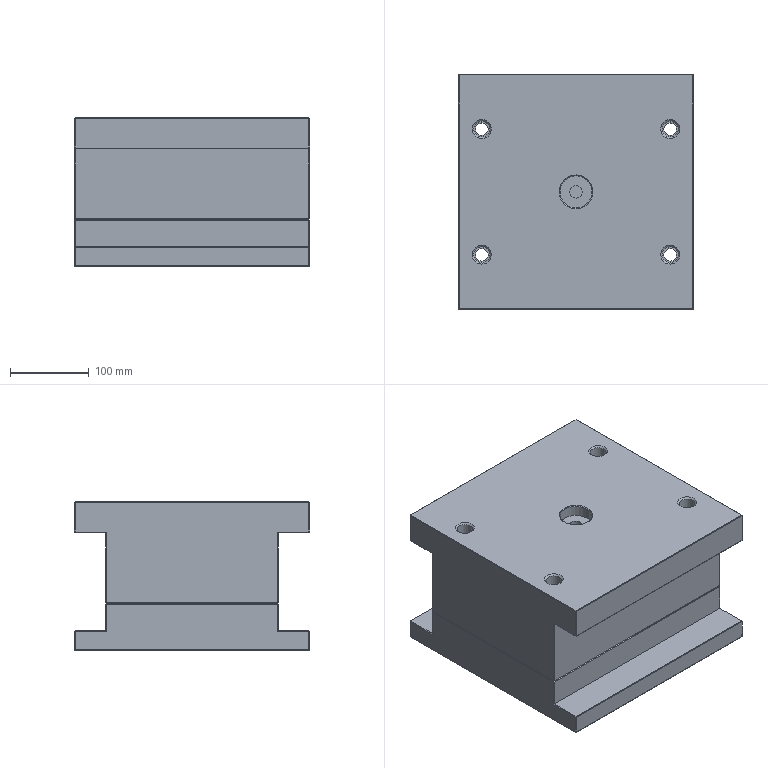NC program | NX | posted with a generic post | part box 300 x 300 x 190 mm
Lines 1 to 898 of 6235:
N10 G17 G21 G94 G90
(CAVITY_MILL , TOOL : D25R5)
N12 T02 M6
N14 G54
N16 G17 G0 G90 X-9.973 Y-6.502 S1000 M3
N18 G43 Z30. H2
N20 Z1.5
N22 G94 G1 X-9.815 Y-6.752 Z1.484 F1000.
N24 X-8.984 Y-7.824 Z1.413
N26 X-8.037 Y-8.794 Z1.342
N28 X-6.985 Y-9.651 Z1.271
N30 X-5.843 Y-10.382 Z1.2
N32 X-4.625 Y-10.979 Z1.129
N34 X-3.347 Y-11.434 Z1.058
N36 X-2.026 Y-11.74 Z0.987
N38 X-0.678 Y-11.894 Z0.916
N40 X0.678 Z0.845
N42 X2.026 Y-11.74 Z0.774
N44 X3.347 Y-11.434 Z0.703
N46 X4.625 Y-10.979 Z0.631
N48 X5.843 Y-10.382 Z0.56
N50 X6.985 Y-9.651 Z0.489
N52 X8.037 Y-8.794 Z0.418
N54 X8.984 Y-7.824 Z0.347
N56 X9.815 Y-6.752 Z0.276
N58 X10.335 Y-5.926 Z0.225
N60 X10.855 Y-4.909 Z0.165
N62 X11.276 Y-3.847 Z0.105
N64 X11.592 Y-2.749 Z0.045
N66 X11.802 Y-1.626 Z-0.015
N68 X11.904 Y-0.488 Z-0.074
N70 Y0. Z-0.1
N72 X2.154
N74 G3 X0. Y2.154 R2.154 F2000.
N76 X2.154 Y0. R-2.154
N78 G1 X11.904
N80 G3 X0. Y11.904 R11.904
N82 X11.904 Y0. R-11.904
N84 G1 X21.654
N86 G3 X0. Y21.654 R21.654
N88 X21.654 Y0. R-21.654
N90 G1 X31.404
N92 G3 X0. Y31.404 R31.404
N94 X31.404 Y0. R-31.404
N96 G1 X41.154
N98 G3 X0. Y41.154 R41.154
N100 X41.154 Y0. R-41.154
N102 X40.654 Y0.866 R1.
N104 G1 Z1.4
N106 G0 X-1.355 Y11.092
N108 G1 X-1.643 Y11.061 Z1.385 F1000.
N110 X-2.887 Y10.804 Z1.318
N112 X-4.095 Y10.406 Z1.252
N114 X-5.249 Y9.874 Z1.185
N116 X-6.336 Y9.215 Z1.118
N118 X-7.341 Y8.436 Z1.052
N120 X-8.251 Y7.549 Z0.985
N122 X-9.054 Y6.564 Z0.919
N124 X-9.74 Y5.494 Z0.852
N126 X-10.301 Y4.353 Z0.785
N128 X-10.728 Y3.156 Z0.719
N130 X-11.017 Y1.918 Z0.652
N132 X-11.164 Y0.655 Z0.585
N134 X-11.166 Y-0.616 Z0.519
N136 X-11.024 Y-1.879 Z0.452
N138 X-10.739 Y-3.118 Z0.386
N140 X-10.316 Y-4.317 Z0.319
N142 X-9.759 Y-5.46 Z0.252
N144 X-9.263 Y-6.265 Z0.203
N146 X-8.471 Y-7.301 Z0.134
N148 X-7.563 Y-8.238 Z0.066
N150 X-6.552 Y-9.062 Z-0.002
N152 X-5.452 Y-9.764 Z-0.071
N154 X-4.277 Y-10.332 Z-0.139
N156 X-3.045 Y-10.76 Z-0.207
N158 X-1.771 Y-11.042 Z-0.276
N160 X-0.473 Y-11.173 Z-0.344
N162 X0. Z-0.369
N164 Y-1.423
N166 G3 X1.423 Y0. R1.423 F2000.
N168 X0. Y-1.423 R-1.423
N170 G1 Y-11.173
N172 G3 X11.173 Y0. R11.173
N174 X0. Y-11.173 R-11.173
N176 G1 Y-20.923
N178 G3 X20.923 Y0. R20.923
N180 X0. Y-20.923 R-20.923
N182 G1 Y-30.673
N184 G3 X30.673 Y0. R30.673
N186 X0. Y-30.673 R-30.673
N188 G1 Y-40.423
N190 G3 X40.423 Y0. R40.423
N192 X0. Y-40.423 R-40.423
N194 X0.866 Y-39.923 R1.
N196 G1 Z1.131
N198 G0 X0.232 Y10.67
N200 G1 X0.115 Y10.676 Z1.125 F1000.
N202 X-0.674 Y10.655 Z1.083
N204 X-1.593 Y10.557 Z1.035
N206 X-2.857 Y10.287 Z0.967
N208 X-4.079 Y9.867 Z0.9
N210 X-5.241 Y9.302 Z0.832
N212 X-6.326 Y8.6 Z0.764
N214 X-7.319 Y7.773 Z0.696
N216 X-8.205 Y6.832 Z0.629
N218 X-8.97 Y5.79 Z0.561
N220 X-9.604 Y4.664 Z0.493
N222 X-10.097 Y3.469 Z0.425
N224 X-10.442 Y2.224 Z0.358
N226 X-10.635 Y0.946 Z0.29
N228 X-10.671 Y-0.346 Z0.222
N230 X-10.551 Y-1.633 Z0.155
N232 X-10.276 Y-2.895 Z0.087
N234 X-9.851 Y-4.116 Z0.019
N236 X-9.282 Y-5.276 Z-0.049
N238 X-8.791 Y-6.059 Z-0.097
N240 X-8.034 Y-7.032 Z-0.162
N242 X-7.17 Y-7.911 Z-0.226
N244 X-6.211 Y-8.684 Z-0.291
N246 X-5.168 Y-9.342 Z-0.355
N248 X-4.057 Y-9.876 Z-0.42
N250 X-2.892 Y-10.277 Z-0.485
N252 X-1.688 Y-10.542 Z-0.549
N254 X-0.462 Y-10.667 Z-0.614
N256 X0. Z-0.638
N258 Y-0.917
N260 G3 X0.917 Y0. R0.917 F2000.
N262 X0. Y-0.917 R-0.917
N264 G1 Y-10.667
N266 G3 X10.667 Y0. R10.667
N268 X0. Y-10.667 R-10.667
N270 G1 Y-20.417
N272 G3 X20.417 Y0. R20.417
N274 X0. Y-20.417 R-20.417
N276 G1 Y-30.167
N278 G3 X30.167 Y0. R30.167
N280 X0. Y-30.167 R-30.167
N282 G1 Y-39.917
N284 G3 X39.917 Y0. R39.917
N286 X0. Y-39.917 R-39.917
N288 X0.866 Y-39.417 R1.
N290 G1 Z0.862
N292 G0 X10.171 Y-1.473
N294 G1 X10.277 Y-0.246 Z0.797 F1000.
N296 X10.228 Y1.034 Z0.73
N298 X10.02 Y2.297 Z0.663
N300 X9.657 Y3.524 Z0.596
N302 X9.144 Y4.697 Z0.529
N304 X8.489 Y5.797 Z0.462
N306 X7.703 Y6.808 Z0.395
N308 X6.797 Y7.712 Z0.328
N310 X5.786 Y8.497 Z0.261
N312 X4.685 Y9.15 Z0.194
N314 X3.511 Y9.662 Z0.126
N316 X2.283 Y10.023 Z0.059
N318 X1.391 Y10.185 Z0.012
N320 X0.464 Y10.269 Z-0.037
N322 X-0.467 Z-0.086
N324 X-1.37 Y10.188 Z-0.133
N326 X-2.541 Y9.961 Z-0.196
N328 X-3.677 Y9.6 Z-0.258
N330 X-4.765 Y9.109 Z-0.321
N332 X-5.788 Y8.496 Z-0.383
N334 X-6.733 Y7.768 Z-0.446
N336 X-7.587 Y6.936 Z-0.508
N338 X-8.339 Y6.011 Z-0.571
N340 X-8.979 Y5.004 Z-0.633
N342 X-9.499 Y3.931 Z-0.696
N344 X-9.89 Y2.804 Z-0.758
N346 X-10.148 Y1.64 Z-0.821
N348 X-10.27 Y0.453 Z-0.883
N350 Y0. Z-0.907
N352 X-0.52
N354 G3 X0. Y-0.52 R0.52 F2000.
N356 X-0.52 Y0. R-0.52
N358 G1 X-10.27
N360 G3 X0. Y-10.27 R10.27
N362 X-10.27 Y0. R-10.27
N364 G1 X-20.02
N366 G3 X0. Y-20.02 R20.02
N368 X-20.02 Y0. R-20.02
N370 G1 X-29.77
N372 G3 X0. Y-29.77 R29.77
N374 X-29.77 Y0. R-29.77
N376 G1 X-39.52
N378 G3 X0. Y-39.52 R39.52
N380 X-39.52 Y0. R-39.52
N382 X-39.02 Y-0.866 R1.
N384 G1 Z0.593
N386 G0 X-11.138 Y0.268
N388 G1 X-11.132 Y-0.701 Z0.542 F1000.
N390 X-10.981 Y-1.958 Z0.476
N392 X-10.689 Y-3.189 Z0.41
N394 X-10.259 Y-4.379 Z0.343
N396 X-9.697 Y-5.513 Z0.277
N398 X-9.196 Y-6.314 Z0.227
N400 X-8.418 Y-7.319 Z0.161
N402 X-7.53 Y-8.229 Z0.094
N404 X-6.545 Y-9.032 Z0.028
N406 X-5.475 Y-9.718 Z-0.039
N408 X-4.334 Y-10.278 Z-0.106
N410 X-3.137 Y-10.704 Z-0.172
N412 X-1.898 Y-10.992 Z-0.239
N414 X-0.636 Y-11.136 Z-0.305
N416 X0.636 Z-0.372
N418 X1.898 Y-10.992 Z-0.439
N420 X3.137 Y-10.704 Z-0.505
N422 X4.334 Y-10.278 Z-0.572
N424 X5.475 Y-9.718 Z-0.639
N426 X6.545 Y-9.032 Z-0.705
N428 X7.53 Y-8.229 Z-0.772
N430 X8.418 Y-7.319 Z-0.838
N432 X9.196 Y-6.314 Z-0.905
N434 X9.697 Y-5.513 Z-0.955
N436 X10.281 Y-4.326 Z-1.024
N438 X10.721 Y-3.079 Z-1.093
N440 X11.01 Y-1.788 Z-1.162
N442 X11.144 Y-0.472 Z-1.232
N444 Y0. Z-1.257
N446 X1.394
N448 G3 X0. Y1.394 R1.394 F2000.
N450 X1.394 Y0. R-1.394
N452 G1 X11.144
N454 G3 X0. Y11.144 R11.144
N456 X11.144 Y0. R-11.144
N458 G1 X20.894
N460 G3 X0. Y20.894 R20.894
N462 X20.894 Y0. R-20.894
N464 G1 X30.644
N466 G3 X0. Y30.644 R30.644
N468 X30.644 Y0. R-30.644
N470 X30.144 Y0.866 R1.
N472 G1 Z0.243
N474 G0 X2.507 Y10.109
N476 G1 X1.744 Y10.286 Z0.202 F1000.
N478 X0.838 Y10.399 Z0.155
N480 X0.154 Y10.432 Z0.119
N482 X-0.53 Y10.419 Z0.083
N484 X-1.44 Y10.333 Z0.035
N486 X-2.676 Y10.084 Z-0.031
N488 X-3.873 Y9.687 Z-0.097
N490 X-5.013 Y9.149 Z-0.163
N492 X-6.081 Y8.477 Z-0.229
N494 X-7.059 Y7.682 Z-0.296
N496 X-7.934 Y6.774 Z-0.362
N498 X-8.694 Y5.767 Z-0.428
N500 X-9.326 Y4.676 Z-0.494
N502 X-9.822 Y3.517 Z-0.56
N504 X-10.175 Y2.306 Z-0.626
N506 X-10.379 Y1.062 Z-0.692
N508 X-10.431 Y-0.198 Z-0.758
N510 X-10.331 Y-1.455 Z-0.824
N512 X-10.08 Y-2.691 Z-0.89
N514 X-9.681 Y-3.888 Z-0.956
N516 X-9.142 Y-5.027 Z-1.023
N518 X-8.667 Y-5.808 Z-1.07
N520 X-7.929 Y-6.78 Z-1.134
N522 X-7.083 Y-7.66 Z-1.198
N524 X-6.14 Y-8.435 Z-1.262
N526 X-5.112 Y-9.094 Z-1.326
N528 X-4.015 Y-9.629 Z-1.39
N530 X-2.863 Y-10.032 Z-1.454
N532 X-1.671 Y-10.298 Z-1.518
N534 X-0.457 Y-10.423 Z-1.582
N536 X0. Z-1.606
N538 Y-0.673
N540 G3 X0.673 Y0. R0.673 F2000.
N542 X0. Y-0.673 R-0.673
N544 G1 Y-10.423
N546 G3 X10.423 Y0. R10.423
N548 X0. Y-10.423 R-10.423
N550 G1 Y-20.173
N552 G3 X20.173 Y0. R20.173
N554 X0. Y-20.173 R-20.173
N556 G1 Y-29.923
N558 G3 X29.923 Y0. R29.923
N560 X0. Y-29.923 R-29.923
N562 X0.866 Y-29.423 R1.
N564 G1 Z-0.106
N566 G0 X4.043 Y9.031
N568 G1 X3.288 Y9.351 Z-0.149 F1000.
N570 X2.1 Y9.687 Z-0.214
N572 X1.223 Y9.836 Z-0.26
N574 X0.358 Y9.906 Z-0.306
N576 X-0.509 Y9.899 Z-0.351
N578 X-1.395 Y9.813 Z-0.398
N580 X-2.573 Y9.572 Z-0.461
N582 X-3.713 Y9.19 Z-0.524
N584 X-4.799 Y8.673 Z-0.587
N586 X-5.814 Y8.028 Z-0.65
N588 X-6.743 Y7.265 Z-0.713
N590 X-7.573 Y6.395 Z-0.776
N592 X-8.292 Y5.431 Z-0.839
N594 X-8.888 Y4.387 Z-0.902
N596 X-9.354 Y3.279 Z-0.965
N598 X-9.682 Y2.122 Z-1.028
N600 X-9.868 Y0.934 Z-1.091
N602 X-9.909 Y-0.267 Z-1.154
N604 X-9.803 Y-1.465 Z-1.217
N606 X-9.554 Y-2.641 Z-1.28
N608 X-9.164 Y-3.779 Z-1.343
N610 X-8.639 Y-4.86 Z-1.406
N612 X-8.168 Y-5.616 Z-1.453
N614 X-7.467 Y-6.519 Z-1.513
N616 X-6.666 Y-7.336 Z-1.573
N618 X-5.777 Y-8.055 Z-1.633
N620 X-4.81 Y-8.667 Z-1.693
N622 X-3.78 Y-9.163 Z-1.753
N624 X-2.699 Y-9.537 Z-1.812
N626 X-1.583 Y-9.785 Z-1.872
N628 X-0.445 Y-9.902 Z-1.932
N630 X0. Z-1.956
N632 Y-0.152
N634 G3 X0.152 Y0. R0.152 F2000.
N636 X0. Y-0.152 R-0.152
N638 G1 Y-9.902
N640 G3 X9.902 Y0. R9.902
N642 X0. Y-9.902 R-9.902
N644 G1 Y-19.652
N646 G3 X19.652 Y0. R19.652
N648 X0. Y-19.652 R-19.652
N650 G1 Y-29.402
N652 G3 X29.402 Y0. R29.402
N654 X0. Y-29.402 R-29.402
N656 X0.866 Y-28.902 R1.
N658 G1 Z-0.456
N660 G0 X7.968 Y-5.164
N662 G1 X8.328 Y-4.575 Z-0.492 F1000.
N664 X8.847 Y-3.466 Z-0.556
N666 X9.219 Y-2.3 Z-0.62
N668 X9.438 Y-1.096 Z-0.684
N670 X9.501 Y0.127 Z-0.748
N672 X9.406 Y1.347 Z-0.813
N674 X9.155 Y2.546 Z-0.877
N676 X8.751 Y3.701 Z-0.941
N678 X8.203 Y4.796 Z-1.005
N680 X7.518 Y5.811 Z-1.069
N682 X6.709 Y6.729 Z-1.133
N684 X5.788 Y7.536 Z-1.198
N686 X4.771 Y8.217 Z-1.262
N688 X3.675 Y8.762 Z-1.326
N690 X2.518 Y9.162 Z-1.39
N692 X1.668 Y9.354 Z-1.436
N694 X0.475 Y9.49 Z-1.499
N696 X-0.725 Y9.474 Z-1.562
N698 X-1.59 Y9.368 Z-1.607
N700 X-2.73 Y9.101 Z-1.669
N702 X-3.829 Y8.696 Z-1.73
N704 X-4.87 Y8.159 Z-1.791
N706 X-5.837 Y7.498 Z-1.853
N708 X-6.715 Y6.723 Z-1.914
N710 X-7.491 Y5.845 Z-1.975
N712 X-8.153 Y4.879 Z-2.037
N714 X-8.692 Y3.839 Z-2.098
N716 X-9.098 Y2.741 Z-2.16
N718 X-9.366 Y1.6 Z-2.221
N720 X-9.492 Y0.436 Z-2.282
N722 Y0. Z-2.305
N724 G3 X-8.01 Y-5.092 R9.492 F2000.
N726 G1 X0. Y0.
N728 X-8.01 Y-5.092
N730 G3 X-9.492 Y0. R-9.492
N732 G1 X-19.242
N734 G3 X0. Y-19.242 R19.242
N736 X-19.242 Y0. R-19.242
N738 G1 X-28.992
N740 G3 X0. Y-28.992 R28.992
N742 X-28.992 Y0. R-28.992
N744 X-28.492 Y-0.866 R1.
N746 G1 Z-0.805
N748 G0 X-6.931 Y5.97
N750 G1 X-7.264 Y5.591 Z-0.832 F1000.
N752 X-7.919 Y4.616 Z-0.893
N754 X-8.444 Y3.566 Z-0.955
N756 X-8.831 Y2.457 Z-1.016
N758 X-9.073 Y1.308 Z-1.078
N760 X-9.165 Y0.137 Z-1.139
N762 X-9.108 Y-1.036 Z-1.201
N764 X-8.901 Y-2.192 Z-1.263
N766 X-8.547 Y-3.312 Z-1.324
N768 X-8.054 Y-4.378 Z-1.386
N770 X-7.61 Y-5.11 Z-1.43
N772 X-6.892 Y-6.044 Z-1.492
N774 X-6.059 Y-6.878 Z-1.554
N776 X-5.127 Y-7.599 Z-1.616
N778 X-4.109 Y-8.194 Z-1.678
N780 X-3.024 Y-8.653 Z-1.739
N782 X-1.889 Y-8.97 Z-1.801
N784 X-0.722 Y-9.138 Z-1.863
N786 X0.456 Y-9.155 Z-1.925
N788 X1.627 Y-9.021 Z-1.986
N790 X2.771 Y-8.738 Z-2.048
N792 X3.869 Y-8.31 Z-2.11
N794 X4.903 Y-7.745 Z-2.172
N796 X5.856 Y-7.052 Z-2.233
N798 X6.713 Y-6.242 Z-2.295
N800 X7.458 Y-5.329 Z-2.357
N802 X7.923 Y-4.61 Z-2.402
N804 X8.418 Y-3.628 Z-2.459
N806 X8.792 Y-2.593 Z-2.517
N808 X9.039 Y-1.522 Z-2.575
N810 X9.156 Y-0.428 Z-2.632
N812 Y0. Z-2.655
N814 G3 X7.691 Y-4.97 R-9.156 F2000.
N816 G1 X0. Y0.
N818 X7.691 Y-4.97
N820 G3 X9.156 Y0. R9.156
N822 G1 X18.906
N824 G3 X0. Y18.906 R18.906
N826 X18.906 Y0. R-18.906
N828 G1 X28.656
N830 G3 X0. Y28.656 R28.656
N832 X28.656 Y0. R-28.656
N834 X28.156 Y0.866 R1.
N836 G1 Z-1.155
N838 G0 X6.56 Y5.976
N840 G1 X6.375 Y6.192 Z-1.17 F1000.
N842 X5.53 Y6.958 Z-1.229
N844 X4.594 Y7.608 Z-1.289
N846 X3.582 Y8.134 Z-1.349
N848 X2.511 Y8.526 Z-1.409
N850 X1.692 Y8.725 Z-1.453
N852 X0.618 Y8.866 Z-1.51
N854 X-0.465 Y8.875 Z-1.566
N856 X-1.304 Y8.791 Z-1.611
N858 X-2.419 Y8.552 Z-1.67
N860 X-3.495 Y8.172 Z-1.73
N862 X-4.513 Y7.657 Z-1.79
N864 X-5.456 Y7.016 Z-1.85
N866 X-6.31 Y6.259 Z-1.91
N868 X-7.06 Y5.399 Z-1.969
N870 X-7.693 Y4.45 Z-2.029
N872 X-8.2 Y3.428 Z-2.089
N874 X-8.571 Y2.35 Z-2.149
N876 X-8.802 Y1.232 Z-2.208
N878 X-8.887 Y0.095 Z-2.268
N880 X-8.826 Y-1.044 Z-2.328
N882 X-8.62 Y-2.166 Z-2.388
N884 X-8.271 Y-3.253 Z-2.448
N886 X-7.786 Y-4.285 Z-2.507
N888 X-7.345 Y-5.004 Z-2.552
N890 X-6.622 Y-5.928 Z-2.613
N892 X-5.783 Y-6.749 Z-2.675
N894 X-4.842 Y-7.453 Z-2.736
N896 X-3.818 Y-8.026 Z-2.798
N898 X-2.727 Y-8.459 Z-2.859
N900 X-1.588 Y-8.745 Z-2.921
N902 X-0.421 Y-8.878 Z-2.982
N904 X0. Z-3.004
N906 G3 X-7.566 Y-4.644 R-8.878 F2000.
N908 G1 X0. Y0.
N910 X-7.566 Y-4.644
N912 G3 X0. Y-8.878 R8.878
N914 G1 Y-18.628
N916 G3 X18.628 Y0. R18.628
N918 X0. Y-18.628 R-18.628
N920 G1 Y-28.378
N922 G3 X28.378 Y0. R28.378
N924 X0. Y-28.378 R-28.378
N926 X0.866 Y-27.878 R1.
N928 G1 Z-1.504
N930 G0 X6.972 Y5.103
N932 G1 X6.796 Y5.358 Z-1.521 F1000.
N934 X6.04 Y6.198 Z-1.58
N936 X5.182 Y6.931 Z-1.639
N938 X4.235 Y7.547 Z-1.698
N940 X3.217 Y8.034 Z-1.757
N942 X2.143 Y8.385 Z-1.817
N944 X1.328 Y8.552 Z-1.86
N946 X0.439 Y8.643 Z-1.907
N948 X-0.455 Y8.642 Z-1.954
N950 X-1.282 Y8.559 Z-1.997
N952 X-2.37 Y8.324 Z-2.056
N954 X-3.418 Y7.951 Z-2.114
N956 X-4.41 Y7.447 Z-2.172
N958 X-5.329 Y6.819 Z-2.231
N960 X-6.159 Y6.079 Z-2.289
N962 X-6.889 Y5.239 Z-2.347
N964 X-7.504 Y4.312 Z-2.406
N966 X-7.995 Y3.314 Z-2.464
N968 X-8.354 Y2.261 Z-2.522
N970 X-8.575 Y1.17 Z-2.58
N972 X-8.654 Y0.061 Z-2.639
N974 X-8.59 Y-1.05 Z-2.697
N976 X-8.385 Y-2.144 Z-2.755
N978 X-8.04 Y-3.202 Z-2.814
N980 X-7.563 Y-4.207 Z-2.872
N982 X-7.125 Y-4.913 Z-2.916
N984 X-6.42 Y-5.804 Z-2.975
N986 X-5.605 Y-6.594 Z-3.035
N988 X-4.694 Y-7.271 Z-3.094
N990 X-3.701 Y-7.823 Z-3.154
N992 X-2.645 Y-8.24 Z-3.213
N994 X-1.544 Y-8.516 Z-3.273
N996 X-0.416 Y-8.644 Z-3.332
N998 X0. Z-3.354
N1000 G3 X-7.344 Y-4.56 R-8.644 F2000.
N1002 G1 X0. Y0.
N1004 X-7.344 Y-4.56
N1006 G3 X0. Y-8.644 R8.644
N1008 G1 Y-18.394
N1010 G3 X18.394 Y0. R18.394
N1012 X0. Y-18.394 R-18.394
N1014 G1 Y-28.144
N1016 G3 X28.144 Y0. R28.144
N1018 X0. Y-28.144 R-28.144
N1020 X0.866 Y-27.644 R1.
N1022 G1 Z-1.854
N1024 G0 X7.257 Y4.33
N1026 G1 X7.183 Y4.469 Z-1.862 F1000.
N1028 X6.525 Y5.385 Z-1.921
N1030 X5.75 Y6.205 Z-1.98
N1032 X4.873 Y6.915 Z-2.04
N1034 X3.909 Y7.502 Z-2.099
N1036 X2.876 Y7.956 Z-2.158
N1038 X1.792 Y8.268 Z-2.217
N1040 X0.98 Y8.403 Z-2.26
N1042 X0.268 Y8.456 Z-2.298
N1044 X-0.446 Y8.448 Z-2.335
N1046 X-1.264 Y8.365 Z-2.378
N1048 X-2.328 Y8.133 Z-2.435
N1050 X-3.354 Y7.767 Z-2.492
N1052 X-4.323 Y7.272 Z-2.549
N1054 X-5.222 Y6.656 Z-2.606
N1056 X-6.033 Y5.93 Z-2.663
N1058 X-6.745 Y5.106 Z-2.72
N1060 X-7.345 Y4.197 Z-2.778
N1062 X-7.824 Y3.219 Z-2.835
N1064 X-8.172 Y2.187 Z-2.892
N1066 X-8.385 Y1.119 Z-2.949
N1068 X-8.46 Y0.033 Z-3.006
N1070 X-8.394 Y-1.054 Z-3.063
N1072 X-8.189 Y-2.124 Z-3.12
N1074 X-7.848 Y-3.158 Z-3.177
N1076 X-7.378 Y-4.14 Z-3.234
N1078 X-6.941 Y-4.837 Z-3.277
N1080 X-6.252 Y-5.699 Z-3.335
N1082 X-5.458 Y-6.464 Z-3.393
N1084 X-4.57 Y-7.119 Z-3.451
N1086 X-3.605 Y-7.654 Z-3.508
N1088 X-2.578 Y-8.058 Z-3.566
N1090 X-1.507 Y-8.324 Z-3.624
N1092 X-0.411 Y-8.45 Z-3.682
N1094 X0. Z-3.703
N1096 G3 X-7.159 Y-4.488 R-8.45 F2000.
N1098 G1 X0. Y0.
N1100 X-7.159 Y-4.488
N1102 G3 X0. Y-8.45 R8.45
N1104 G1 Y-18.2
N1106 G3 X18.2 Y0. R18.2
N1108 X0. Y-18.2 R-18.2
N1110 G1 Y-27.95
N1112 G3 X27.95 Y0. R27.95
N1114 X0. Y-27.95 R-27.95
N1116 X0.866 Y-27.45 R1.
N1118 G1 Z-2.203
N1120 G0 X7.441 Y3.658
N1122 G1 X6.954 Y4.53 Z-2.256 F1000.
N1124 X6.272 Y5.434 Z-2.315
N1126 X5.475 Y6.237 Z-2.375
N1128 X4.575 Y6.924 Z-2.434
N1130 X3.59 Y7.482 Z-2.493
N1132 X2.539 Y7.901 Z-2.552
N1134 X1.44 Y8.173 Z-2.612
N1136 X0.632 Y8.275 Z-2.654
N1138 X0. Y8.299 Z-2.688
N1140 X-0.632 Y8.275 Z-2.721
N1142 X-1.44 Y8.173 Z-2.763
N1144 X-2.539 Y7.901 Z-2.823
N1146 X-3.59 Y7.482 Z-2.882
N1148 X-4.575 Y6.924 Z-2.941
N1150 X-5.475 Y6.237 Z-3.001
N1152 X-6.272 Y5.434 Z-3.06
N1154 X-6.954 Y4.53 Z-3.119
N1156 X-7.505 Y3.542 Z-3.179
N1158 X-7.917 Y2.488 Z-3.238
N1160 X-8.182 Y1.387 Z-3.297
N1162 X-8.295 Y0.261 Z-3.357
N1164 X-8.253 Y-0.87 Z-3.416
N1166 X-8.058 Y-1.985 Z-3.475
N1168 X-7.713 Y-3.063 Z-3.535
N1170 X-7.225 Y-4.084 Z-3.594
N1172 X-6.789 Y-4.773 Z-3.637
N1174 X-6.114 Y-5.612 Z-3.693
N1176 X-5.336 Y-6.356 Z-3.75
N1178 X-4.468 Y-6.994 Z-3.806
N1180 X-3.525 Y-7.513 Z-3.862
N1182 X-2.522 Y-7.907 Z-3.919
N1184 X-1.477 Y-8.167 Z-3.975
N1186 X-0.407 Y-8.289 Z-4.032
N1188 X0. Z-4.053
N1190 G3 X-7.007 Y-4.428 R-8.289 F2000.
N1192 G1 X0. Y0.
N1194 X-7.007 Y-4.428
N1196 G3 X0. Y-8.289 R8.289
N1198 G1 Y-18.039
N1200 G3 X18.039 Y0. R18.039
N1202 X0. Y-18.039 R-18.039
N1204 G1 Y-27.789
N1206 G3 X27.789 Y0. R27.789
N1208 X0. Y-27.789 R-27.789
N1210 X0.866 Y-27.289 R1.
N1212 G1 Z-2.553
N1214 G0 X7.541 Y3.091
N1216 G1 X7.352 Y3.561 Z-2.58 F1000.
N1218 X6.79 Y4.541 Z-2.639
N1220 X6.099 Y5.434 Z-2.698
N1222 X5.292 Y6.223 Z-2.757
N1224 X4.383 Y6.893 Z-2.816
N1226 X3.391 Y7.432 Z-2.875
N1228 X2.334 Y7.828 Z-2.935
N1230 X1.549 Y8.021 Z-2.977
N1232 X0.458 Y8.156 Z-3.035
N1234 X-0.642 Y8.144 Z-3.092
N1236 X-1.443 Y8.04 Z-3.135
N1238 X-2.524 Y7.769 Z-3.193
N1240 X-3.557 Y7.354 Z-3.251
N1242 X-4.524 Y6.802 Z-3.31
N1244 X-5.407 Y6.123 Z-3.368
N1246 X-6.19 Y5.331 Z-3.426
N1248 X-6.858 Y4.439 Z-3.485
N1250 X-7.398 Y3.465 Z-3.543
N1252 X-7.8 Y2.426 Z-3.602
N1254 X-8.058 Y1.343 Z-3.66
N1256 X-8.166 Y0.234 Z-3.718
N1258 X-8.122 Y-0.879 Z-3.777
N1260 X-7.927 Y-1.975 Z-3.835
N1262 X-7.584 Y-3.035 Z-3.893
N1264 X-7.101 Y-4.038 Z-3.952
N1266 X-6.667 Y-4.72 Z-3.994
N1268 X-6.003 Y-5.541 Z-4.049
N1270 X-5.238 Y-6.269 Z-4.105
N1272 X-4.386 Y-6.892 Z-4.16
N1274 X-3.461 Y-7.4 Z-4.215
N1276 X-2.477 Y-7.784 Z-4.271
N1278 X-1.453 Y-8.039 Z-4.326
N1280 X-0.404 Y-8.159 Z-4.381
N1282 X0. Z-4.403
N1284 G3 X-6.884 Y-4.379 R-8.159 F2000.
N1286 G1 X0. Y0.
N1288 X-6.884 Y-4.379
N1290 G3 X0. Y-8.159 R8.159
N1292 G1 Y-17.909
N1294 G3 X17.909 Y0. R17.909
N1296 X0. Y-17.909 R-17.909
N1298 G1 Y-27.659
N1300 G3 X27.659 Y0. R27.659
N1302 X0. Y-27.659 R-27.659
N1304 X0.866 Y-27.159 R1.
N1306 G1 Z-2.903
N1308 G0 X-7.604 Y-2.64
N1310 G1 X-7.483 Y-3.012 Z-2.923 F1000.
N1312 X-7.004 Y-4.002 Z-2.981
N1314 X-6.571 Y-4.679 Z-3.023
N1316 X-5.873 Y-5.53 Z-3.081
N1318 X-5.066 Y-6.278 Z-3.138
N1320 X-4.164 Y-6.909 Z-3.196
N1322 X-3.185 Y-7.412 Z-3.254
N1324 X-2.146 Y-7.776 Z-3.311
N1326 X-1.067 Y-7.996 Z-3.369
N1328 X0.031 Y-8.067 Z-3.427
N1330 X1.129 Y-7.987 Z-3.484
N1332 X2.206 Y-7.759 Z-3.542
N1334 X3.242 Y-7.387 Z-3.6
N1336 X4.217 Y-6.877 Z-3.657
N1338 X5.114 Y-6.239 Z-3.715
N1340 X5.916 Y-5.484 Z-3.773
N1342 X6.607 Y-4.628 Z-3.83
N1344 X7.035 Y-3.948 Z-3.873
N1346 X7.514 Y-2.935 Z-3.931
N1348 X7.848 Y-1.865 Z-3.99
N1350 X8.031 Y-0.759 Z-4.049
N1352 X8.059 Y0.361 Z-4.108
N1354 X7.931 Y1.475 Z-4.166
N1356 X7.65 Y2.56 Z-4.225
N1358 X7.221 Y3.596 Z-4.284
N1360 X6.653 Y4.562 Z-4.343
N1362 X5.956 Y5.44 Z-4.401
N1364 X5.145 Y6.213 Z-4.46
N1366 X4.234 Y6.866 Z-4.519
N1368 X3.241 Y7.387 Z-4.577
N1370 X2.186 Y7.765 Z-4.636
N1372 X1.403 Y7.944 Z-4.678
N1374 X0.402 Y8.057 Z-4.731
N1376 X0. Z-4.752
N1378 G3 X-6.788 Y-4.341 R8.057 F2000.
N1380 G1 X0. Y0.
N1382 X-6.788 Y-4.341
N1384 G3 X0. Y8.057 R-8.057
N1386 G1 Y17.807
N1388 G3 X-17.807 Y0. R17.807
N1390 X0. Y17.807 R-17.807
N1392 G1 Y27.557
N1394 G3 X-27.557 Y0. R27.557
N1396 X0. Y27.557 R-27.557
N1398 X-0.866 Y27.057 R1.
N1400 G1 Z-3.252
N1402 G0 X7.638 Y2.302
N1404 G1 X7.576 Y2.541 Z-3.265 F1000.
N1406 X7.145 Y3.578 Z-3.324
N1408 X6.573 Y4.545 Z-3.383
N1410 X5.87 Y5.422 Z-3.442
N1412 X5.052 Y6.191 Z-3.501
N1414 X4.134 Y6.839 Z-3.559
N1416 X3.134 Y7.351 Z-3.618
N1418 X2.072 Y7.718 Z-3.677
N1420 X1.291 Y7.886 Z-3.719
N1422 X0.436 Y7.979 Z-3.764
N1424 X-0.424 Y7.98 Z-3.809
N1426 X-1.219 Y7.897 Z-3.851
N1428 X-2.281 Y7.659 Z-3.908
N1430 X-3.3 Y7.278 Z-3.965
N1432 X-4.258 Y6.762 Z-4.022
N1434 X-5.137 Y6.121 Z-4.079
N1436 X-5.921 Y5.366 Z-4.136
N1438 X-6.596 Y4.512 Z-4.193
N1440 X-7.147 Y3.574 Z-4.25
N1442 X-7.567 Y2.569 Z-4.307
N1444 X-7.846 Y1.517 Z-4.364
N1446 X-7.979 Y0.437 Z-4.421
N1448 X-7.964 Y-0.651 Z-4.478
N1450 X-7.802 Y-1.727 Z-4.536
N1452 X-7.495 Y-2.771 Z-4.593
N1454 X-7.049 Y-3.764 Z-4.65
N1456 X-6.638 Y-4.449 Z-4.691
N1458 X-5.99 Y-5.289 Z-4.747
N1460 X-5.236 Y-6.036 Z-4.803
N1462 X-4.39 Y-6.677 Z-4.858
N1464 X-3.467 Y-7.2 Z-4.914
N1466 X-2.482 Y-7.596 Z-4.97
N1468 X-1.454 Y-7.858 Z-5.025
N1470 X-0.4 Y-7.981 Z-5.081
N1472 X0. Z-5.102
N1474 G3 X6.716 Y-4.312 R7.981 F2000.
N1476 G1 X0. Y0.
N1478 X6.716 Y-4.312
N1480 G3 X0. Y-7.981 R-7.981
N1482 G1 Y-17.731
N1484 G3 X17.731 Y0. R17.731
N1486 X0. Y-17.731 R-17.731
N1488 G1 Y-27.481
N1490 G3 X27.481 Y0. R27.481
N1492 X0. Y-27.481 R-27.481
N1494 X0.866 Y-26.981 R1.
N1496 G1 Z-3.602
N1498 G0 X7.645 Y2.071
N1500 G1 X7.52 Y2.55 Z-3.628 F1000.
N1502 X7.085 Y3.585 Z-3.687
N1504 X6.509 Y4.548 Z-3.745
N1506 X5.803 Y5.42 Z-3.804
N1508 X4.981 Y6.184 Z-3.863
N1510 X4.059 Y6.824 Z-3.922
N1512 X3.057 Y7.329 Z-3.981
N1514 X1.993 Y7.686 Z-4.039
N1516 X1.213 Y7.847 Z-4.081
N1518 X0.398 Y7.93 Z-4.124
N1520 X-0.421 Y7.929 Z-4.167
N1522 X-1.214 Y7.847 Z-4.209
N1524 X-2.269 Y7.609 Z-4.265
N1526 X-3.282 Y7.23 Z-4.322
N1528 X-4.234 Y6.717 Z-4.379
N1530 X-5.108 Y6.079 Z-4.436
N1532 X-5.887 Y5.329 Z-4.492
N1534 X-6.556 Y4.479 Z-4.549
N1536 X-7.104 Y3.546 Z-4.606
N1538 X-7.52 Y2.548 Z-4.662
N1540 X-7.797 Y1.502 Z-4.719
N1542 X-7.929 Y0.428 Z-4.776
N1544 X-7.913 Y-0.653 Z-4.832
N1546 X-7.751 Y-1.723 Z-4.889
N1548 X-7.445 Y-2.76 Z-4.946
N1550 X-7.001 Y-3.746 Z-5.002
N1552 X-6.59 Y-4.429 Z-5.044
N1554 X-5.946 Y-5.262 Z-5.099
N1556 X-5.198 Y-6.003 Z-5.155
N1558 X-4.358 Y-6.638 Z-5.21
N1560 X-3.441 Y-7.156 Z-5.265
N1562 X-2.464 Y-7.548 Z-5.32
N1564 X-1.444 Y-7.808 Z-5.375
N1566 X-0.398 Y-7.93 Z-5.43
N1568 X0. Z-5.451
N1570 G3 X6.668 Y-4.292 R7.93 F2000.
N1572 G1 X0. Y0.
N1574 X6.668 Y-4.292
N1576 G3 X0. Y-7.93 R-7.93
N1578 G1 Y-17.68
N1580 G3 X17.68 Y0. R17.68
N1582 X0. Y-17.68 R-17.68
N1584 G1 Y-27.43
N1586 G3 X27.43 Y0. R27.43
N1588 X0. Y-27.43 R-27.43
N1590 X0.866 Y-26.93 R1.
N1592 G1 Z-3.951
N1594 G0 X7.65 Y1.951
N1596 G1 X7.49 Y2.556 Z-3.984 F1000.
N1598 X7.054 Y3.589 Z-4.043
N1600 X6.475 Y4.55 Z-4.102
N1602 X5.767 Y5.42 Z-4.16
N1604 X4.943 Y6.181 Z-4.219
N1606 X4.02 Y6.817 Z-4.278
N1608 X3.016 Y7.317 Z-4.337
N1610 X1.951 Y7.67 Z-4.396
N1612 X1.171 Y7.827 Z-4.437
N1614 X0.378 Y7.905 Z-4.479
N1616 X-0.42 Y7.903 Z-4.521
N1618 X-1.211 Y7.821 Z-4.562
N1620 X-2.263 Y7.584 Z-4.619
N1622 X-3.273 Y7.206 Z-4.676
N1624 X-4.222 Y6.694 Z-4.732
N1626 X-5.093 Y6.058 Z-4.789
N1628 X-5.869 Y5.309 Z-4.845
N1630 X-6.536 Y4.462 Z-4.902
N1632 X-7.082 Y3.532 Z-4.958
N1634 X-7.497 Y2.537 Z-5.015
N1636 X-7.772 Y1.494 Z-5.071
N1638 X-7.903 Y0.424 Z-5.128
N1640 X-7.887 Y-0.654 Z-5.184
N1642 X-7.725 Y-1.72 Z-5.241
N1644 X-7.419 Y-2.754 Z-5.297
N1646 X-6.976 Y-3.737 Z-5.354
N1648 X-6.566 Y-4.419 Z-5.395
N1650 X-5.924 Y-5.248 Z-5.45
N1652 X-5.178 Y-5.985 Z-5.505
N1654 X-4.341 Y-6.617 Z-5.56
N1656 X-3.428 Y-7.133 Z-5.615
N1658 X-2.455 Y-7.524 Z-5.67
N1660 X-1.439 Y-7.782 Z-5.725
N1662 X-0.398 Y-7.904 Z-5.78
N1664 X0. Z-5.801
N1666 G3 X6.644 Y-4.282 R7.904 F2000.
N1668 G1 X0. Y0.
N1670 X6.644 Y-4.282
N1672 G3 X0. Y-7.904 R-7.904
N1674 G1 Y-17.654
N1676 G3 X17.654 Y0. R17.654
N1678 X0. Y-17.654 R-17.654
N1680 G1 Y-27.404
N1682 G3 X27.404 Y0. R27.404
N1684 X0. Y-27.404 R-27.404
N1686 X0.866 Y-26.904 R1.
N1688 G1 Z-4.301
N1690 G0 X-1.937 Y7.664
N1692 G1 X-2.825 Y7.388 Z-4.35 F1000.
N1694 X-3.746 Y6.967 Z-4.403
N1696 X-4.606 Y6.43 Z-4.456
N1698 X-5.391 Y5.788 Z-4.509
N1700 X-5.945 Y5.218 Z-4.551
N1702 X-6.592 Y4.372 Z-4.606
N1704 X-7.119 Y3.447 Z-4.662
N1706 X-7.518 Y2.46 Z-4.718
N1708 X-7.78 Y1.428 Z-4.774
N1710 X-7.901 Y0.371 Z-4.83
N1712 X-7.88 Y-0.694 Z-4.885
N1714 X-7.715 Y-1.746 Z-4.941
N1716 X-7.411 Y-2.766 Z-4.997
N1718 X-6.972 Y-3.736 Z-5.053
N1720 X-6.562 Y-4.417 Z-5.094
N1722 X-5.894 Y-5.275 Z-5.151
N1724 X-5.115 Y-6.034 Z-5.208
N1726 X-4.239 Y-6.678 Z-5.265
N1728 X-3.283 Y-7.197 Z-5.322
N1730 X-2.265 Y-7.579 Z-5.379
N1732 X-1.204 Y-7.818 Z-5.436
N1734 X-0.12 Y-7.909 Z-5.493
N1736 X0.966 Y-7.851 Z-5.55
N1738 X2.033 Y-7.644 Z-5.607
N1740 X3.062 Y-7.293 Z-5.664
N1742 X4.034 Y-6.804 Z-5.721
N1744 X4.929 Y-6.187 Z-5.778
N1746 X5.731 Y-5.452 Z-5.835
N1748 X6.424 Y-4.615 Z-5.892
N1750 X6.855 Y-3.946 Z-5.934
N1752 X7.272 Y-3.112 Z-5.983
N1754 X7.588 Y-2.234 Z-6.032
N1756 X7.798 Y-1.325 Z-6.081
N1758 X7.9 Y-0.398 Z-6.13
N1760 Y0. Z-6.15
N1762 G3 X1.554 Y7.746 R7.9 F2000.
N1764 G1 X0. Y0.
N1766 X1.554 Y7.746
N1768 G3 X7.9 Y0. R-7.9
N1770 G1 X17.65
N1772 G3 X0. Y17.65 R17.65
N1774 X17.65 Y0. R-17.65
N1776 G1 X27.4
N1778 G3 X0. Y27.4 R27.4
N1780 X27.4 Y0. R-27.4
N1782 X26.9 Y0.866 R1.
N1784 G1 Z-4.65
N1786 G0 X-1.937 Y7.664
N1788 G1 X-2.825 Y7.388 Z-4.699 F1000.
N1790 X-3.746 Y6.967 Z-4.752
N1792 X-4.606 Y6.43 Z-4.805
N1794 X-5.391 Y5.788 Z-4.859